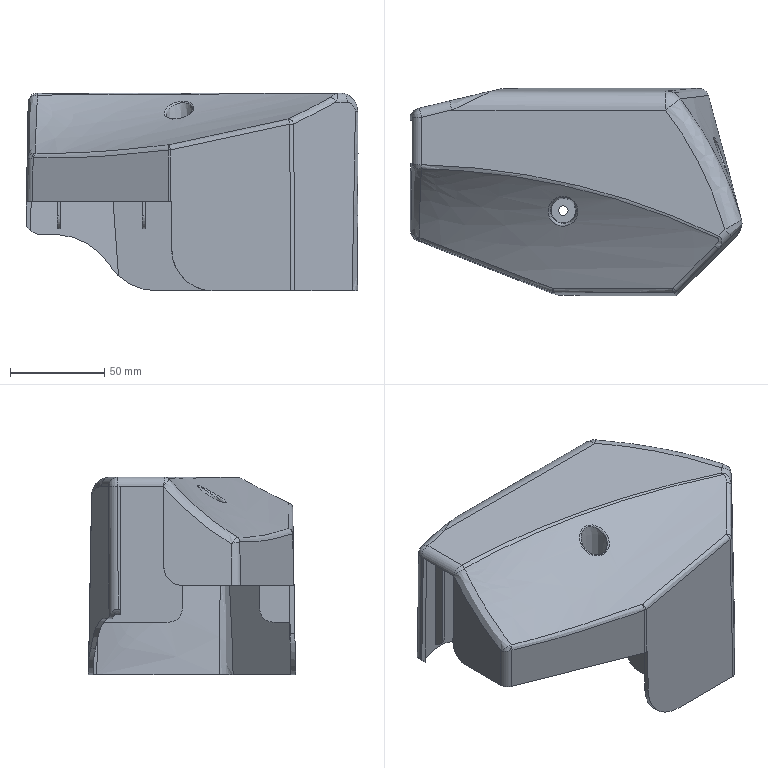Part | STEP file | HHJL | 1 solid | 136 faces | box 176.285 x 110 x 105 mm | volume 139375 mm3 | plane 54 | spline 43 | cylinder 32 | sphere 5 | cone 2 | commonest cylinder face diameters 10 x6 14 x6 15 x5 5 x4 20 x3 1 x2